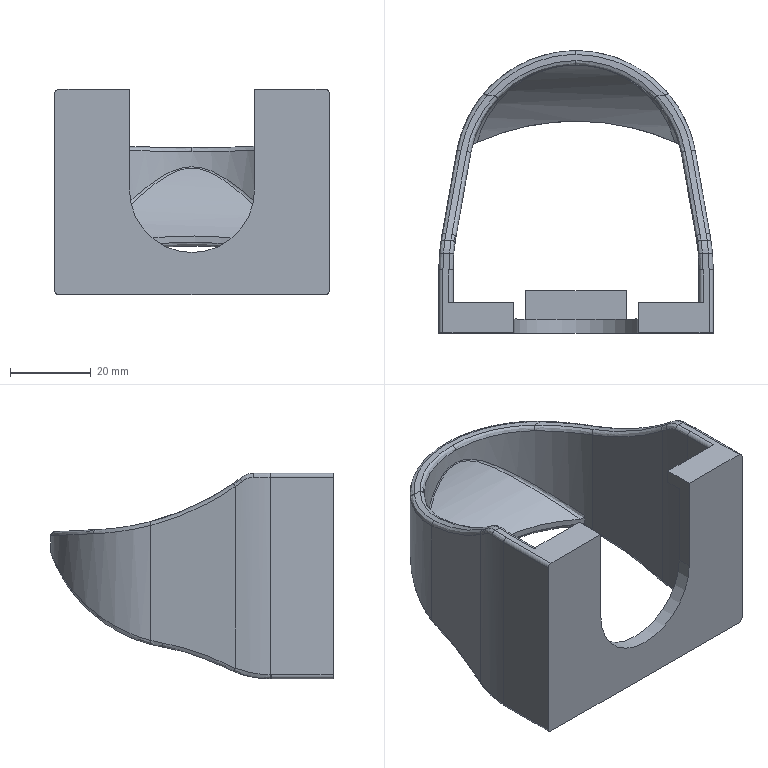Part | SolidWorks | features RefAxis 3, BaseBody 1 | 1 solid | 99 faces | box 68 x 70 x 51 mm | volume 29414 mm3 | spline 49 | cylinder 26 | plane 24 | commonest cylinder face diameters 2 x8 10 x2 51 x2 93 x2 100 x2 110.057 x2